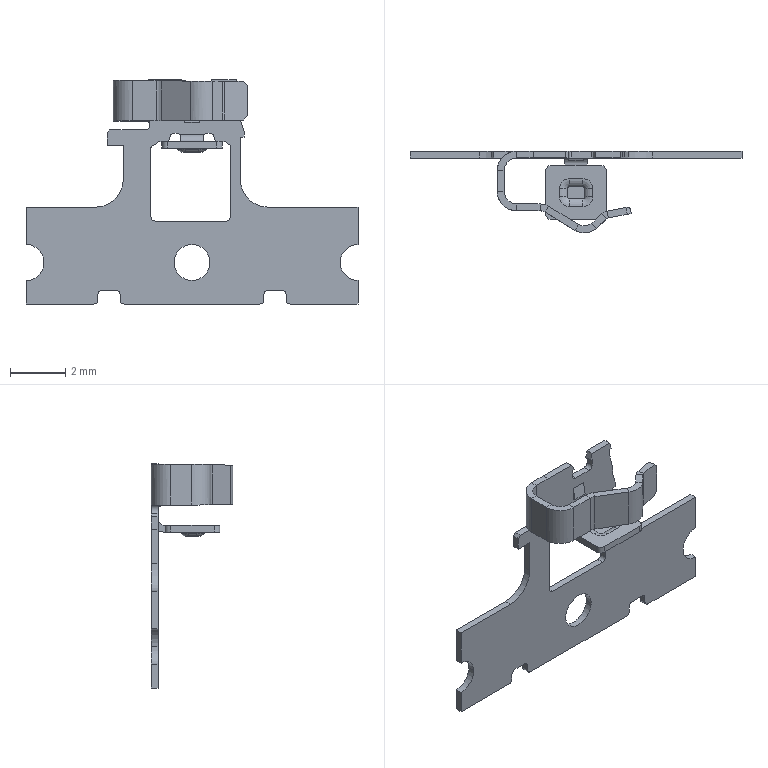Part | NX | 1 solid | 177 faces | box 12 x 2.959 x 8.097 mm | volume 15.937 mm3 | plane 107 | cylinder 56 | torus 12 | spline 2 | commonest cylinder face diameters 0.3 x16 0.2 x6 1.3 x6 0.5 x5 0.7 x5 0.35 x4